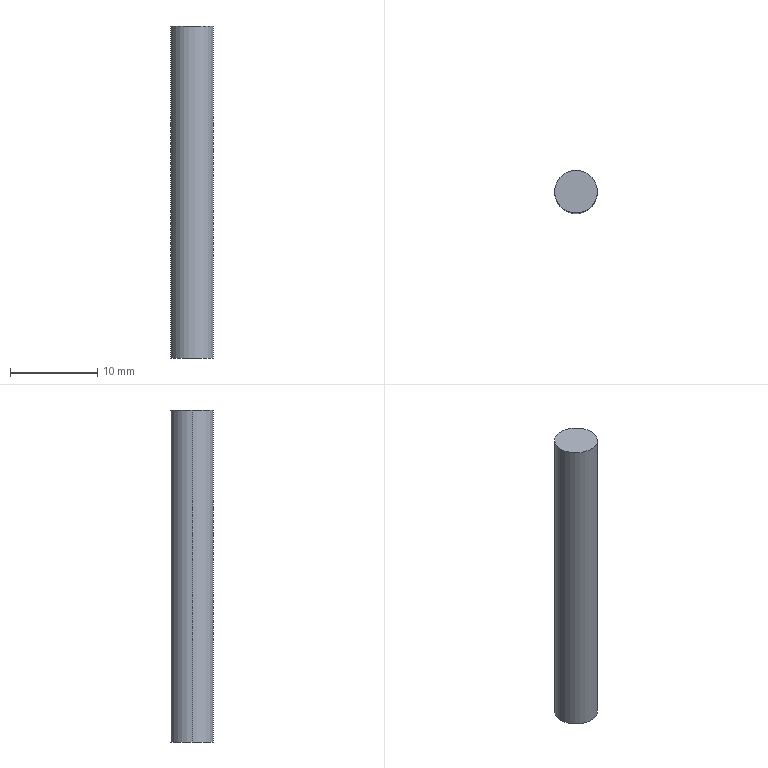Part | SolidWorks | features Extrusion 1 | 1 solid | 4 faces | box 4.9 x 4.9 x 38 mm | volume 716.582 mm3 | cylinder 2 | plane 2 | commonest cylinder face diameters 4.9 x2
STEP:
#1=CARTESIAN_POINT('',(2.45,0.,38.));
#2=VERTEX_POINT('',#1);
#3=CARTESIAN_POINT('',(-2.45,0.,38.));
#4=VERTEX_POINT('',#3);
#5=CARTESIAN_POINT('',(0.,0.,38.));
#6=DIRECTION('',(0.,0.,1.));
#7=DIRECTION('',(1.,0.,0.));
#8=AXIS2_PLACEMENT_3D('',#5,#6,#7);
#9=CIRCLE('',#8,2.45);
#10=EDGE_CURVE('',#2,#4,#9,.T.);
#11=ORIENTED_EDGE('',*,*,#10,.F.);
#12=CARTESIAN_POINT('',(2.45,0.,0.));
#13=VERTEX_POINT('',#12);
#14=CARTESIAN_POINT('',(2.45,0.,38.));
#15=DIRECTION('',(0.,0.,-1.));
#16=VECTOR('',#15,1000.);
#17=LINE('',#14,#16);
#18=EDGE_CURVE('',#2,#13,#17,.T.);
#19=ORIENTED_EDGE('',*,*,#18,.T.);
#20=CARTESIAN_POINT('',(-2.45,0.,0.));
#21=VERTEX_POINT('',#20);
#22=CARTESIAN_POINT('',(0.,0.,0.));
#23=DIRECTION('',(0.,0.,1.));
#24=DIRECTION('',(1.,0.,0.));
#25=AXIS2_PLACEMENT_3D('',#22,#23,#24);
#26=CIRCLE('',#25,2.45);
#27=EDGE_CURVE('',#13,#21,#26,.T.);
#28=ORIENTED_EDGE('',*,*,#27,.T.);
#29=CARTESIAN_POINT('',(-2.45,0.,38.));
#30=DIRECTION('',(0.,0.,-1.));
#31=VECTOR('',#30,1000.);
#32=LINE('',#29,#31);
#33=EDGE_CURVE('',#4,#21,#32,.T.);
#34=ORIENTED_EDGE('',*,*,#33,.F.);
#35=EDGE_LOOP('',(#11,#19,#28,#34));
#36=FACE_OUTER_BOUND('',#35,.T.);
#37=CARTESIAN_POINT('',(0.,0.,38.));
#38=DIRECTION('',(0.,0.,-1.));
#39=DIRECTION('',(-1.,0.,0.));
#40=AXIS2_PLACEMENT_3D('',#37,#38,#39);
#41=CYLINDRICAL_SURFACE('',#40,2.45);
#42=ADVANCED_FACE('',(#36),#41,.T.);
#43=ORIENTED_EDGE('',*,*,#18,.F.);
#44=CARTESIAN_POINT('',(0.,0.,38.));
#45=DIRECTION('',(0.,0.,1.));
#46=DIRECTION('',(1.,0.,0.));
#47=AXIS2_PLACEMENT_3D('',#44,#45,#46);
#48=CIRCLE('',#47,2.45);
#49=EDGE_CURVE('',#4,#2,#48,.T.);
#50=ORIENTED_EDGE('',*,*,#49,.F.);
#51=ORIENTED_EDGE('',*,*,#33,.T.);
#52=CARTESIAN_POINT('',(0.,0.,0.));
#53=DIRECTION('',(0.,0.,1.));
#54=DIRECTION('',(1.,0.,0.));
#55=AXIS2_PLACEMENT_3D('',#52,#53,#54);
#56=CIRCLE('',#55,2.45);
#57=EDGE_CURVE('',#21,#13,#56,.T.);
#58=ORIENTED_EDGE('',*,*,#57,.T.);
#59=EDGE_LOOP('',(#43,#50,#51,#58));
#60=FACE_OUTER_BOUND('',#59,.T.);
#61=CARTESIAN_POINT('',(0.,0.,38.));
#62=DIRECTION('',(0.,0.,-1.));
#63=DIRECTION('',(-1.,0.,0.));
#64=AXIS2_PLACEMENT_3D('',#61,#62,#63);
#65=CYLINDRICAL_SURFACE('',#64,2.45);
#66=ADVANCED_FACE('',(#60),#65,.T.);
#67=ORIENTED_EDGE('',*,*,#49,.T.);
#68=ORIENTED_EDGE('',*,*,#10,.T.);
#69=EDGE_LOOP('',(#67,#68));
#70=FACE_OUTER_BOUND('',#69,.T.);
#71=CARTESIAN_POINT('',(0.,0.,38.));
#72=DIRECTION('',(0.,0.,1.));
#73=DIRECTION('',(1.,0.,0.));
#74=AXIS2_PLACEMENT_3D('',#71,#72,#73);
#75=PLANE('',#74);
#76=ADVANCED_FACE('',(#70),#75,.T.);
#77=ORIENTED_EDGE('',*,*,#57,.F.);
#78=ORIENTED_EDGE('',*,*,#27,.F.);
#79=EDGE_LOOP('',(#77,#78));
#80=FACE_OUTER_BOUND('',#79,.T.);
#81=CARTESIAN_POINT('',(0.,0.,0.));
#82=DIRECTION('',(0.,0.,1.));
#83=DIRECTION('',(1.,0.,0.));
#84=AXIS2_PLACEMENT_3D('',#81,#82,#83);
#85=PLANE('',#84);
#86=ADVANCED_FACE('',(#80),#85,.F.);
#87=CLOSED_SHELL('',(#42,#66,#76,#86));
#88=MANIFOLD_SOLID_BREP('',#87);
#89=CARTESIAN_POINT('',(0.,0.,0.));
#90=DIRECTION('',(0.,0.,1.));
#91=DIRECTION('',(1.,0.,0.));
#92=AXIS2_PLACEMENT_3D('',#89,#90,#91);
#93=(LENGTH_UNIT()NAMED_UNIT(*)SI_UNIT(.MILLI.,.METRE.));
#94=UNCERTAINTY_MEASURE_WITH_UNIT(LENGTH_MEASURE(0.00001),#93,'','');
#95=(NAMED_UNIT(*)PLANE_ANGLE_UNIT()SI_UNIT($,.RADIAN.));
#96=(NAMED_UNIT(*)SI_UNIT($,.STERADIAN.)SOLID_ANGLE_UNIT());
#97=(GEOMETRIC_REPRESENTATION_CONTEXT(3)GLOBAL_UNCERTAINTY_ASSIGNED_CONTEXT((#94))GLOBAL_UNIT_ASSIGNED_CONTEXT((#93,#95,#96))REPRESENTATION_CONTEXT('',''));
#98=ADVANCED_BREP_SHAPE_REPRESENTATION('',(#88,#92),#97);